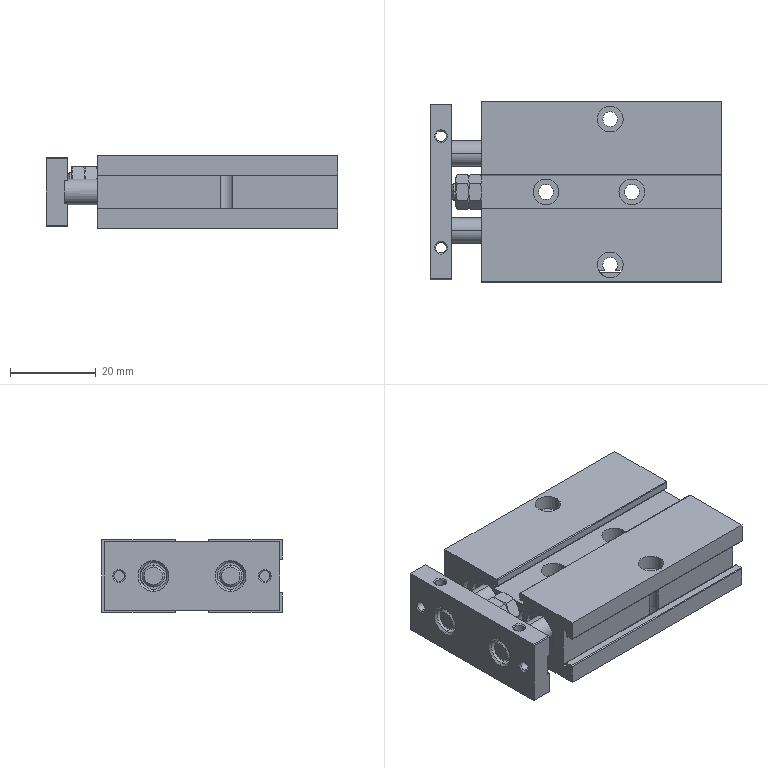Part | SolidWorks | features BaseBody 2, MoveFace 1 | 2 solids | 267 faces | box 68 x 42 x 17 mm | volume 36294 mm3 | cylinder 107 | plane 104 | cone 56 | commonest cylinder face diameters 0.4 x26 6 x24 3.5 x9 2.459 x8 9 x8 10 x8